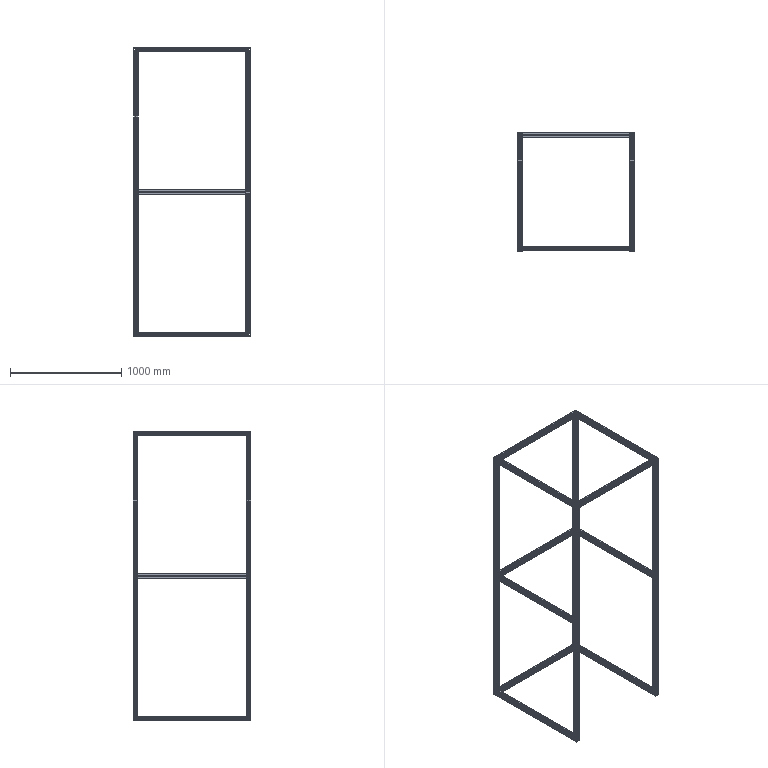Part | SolidWorks | features WeldCornerFeat 3, 3DProfileFeature 1, HoleWzd 1, WeldMemberFeat 1, WeldmentFeature 1 | 14 solids | 1306 faces | box 1050 x 1060 x 2600 mm | volume 7986289 mm3 | plane 964 | cylinder 342 | commonest cylinder face diameters 14 x102 2.2 x84 9 x64 1 x56 15 x36